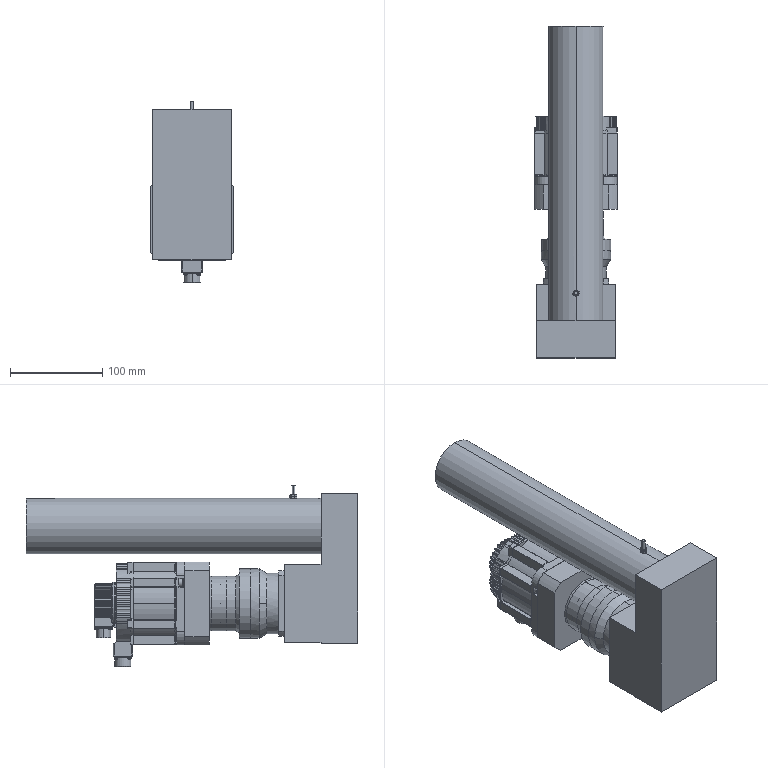Part | STEP file | Base body | 45 solids | 2620 faces | box 90 x 360 x 196.75 mm | volume 2809262 mm3 | cylinder 1180 | plane 820 | torus 329 | cone 177 | sphere 87 | spline 27 | commonest cylinder face diameters 1 x211 2 x102 1.5 x86 0.3 x40 0.5 x40 85 x39